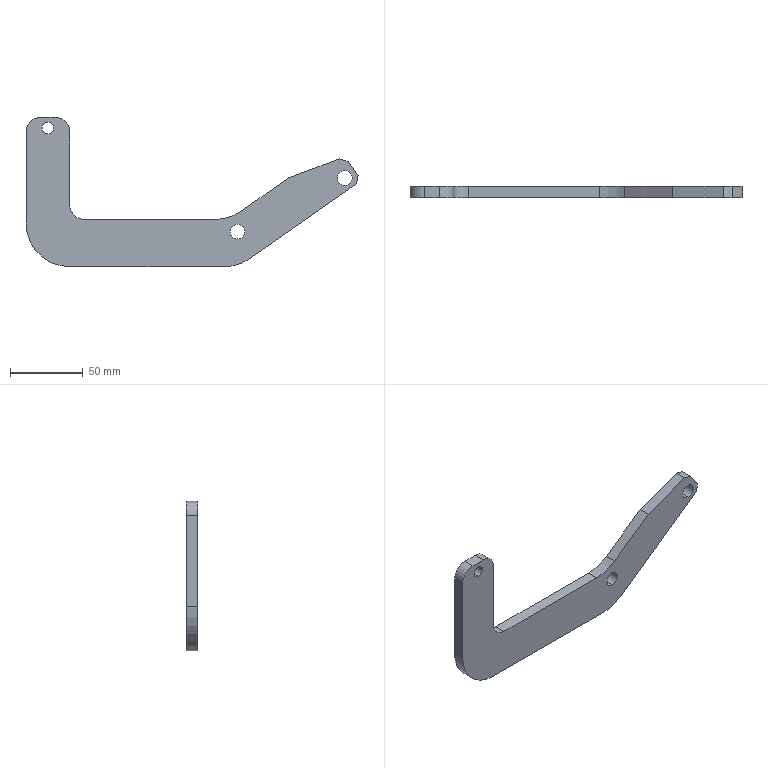Part | SolidWorks | features Extrusion 1, Fillet 1, ICE 1 | 1 solid | 25 faces | box 227.652 x 7.9 x 102.468 mm | volume 70886 mm3 | plane 13 | cylinder 12 | commonest cylinder face diameters 10 x4 20 x3 60 x3 8 x2
STEP:
#1=CARTESIAN_POINT('',(114.715,7.9,3.068));
#2=VERTEX_POINT('',#1);
#3=CARTESIAN_POINT('',(114.715,7.9,-6.932));
#4=VERTEX_POINT('',#3);
#5=CARTESIAN_POINT('',(114.715,7.9,-1.932));
#6=DIRECTION('',(0.,-1.,0.));
#7=DIRECTION('',(0.,0.,-1.));
#8=AXIS2_PLACEMENT_3D('',#5,#6,#7);
#9=CIRCLE('',#8,5.);
#10=EDGE_CURVE('',#2,#4,#9,.T.);
#11=ORIENTED_EDGE('',*,*,#10,.F.);
#12=CARTESIAN_POINT('',(114.715,0.,3.068));
#13=VERTEX_POINT('',#12);
#14=CARTESIAN_POINT('',(114.715,7.9,3.068));
#15=DIRECTION('',(0.,-1.,0.));
#16=VECTOR('',#15,1000.);
#17=LINE('',#14,#16);
#18=EDGE_CURVE('',#2,#13,#17,.T.);
#19=ORIENTED_EDGE('',*,*,#18,.T.);
#20=CARTESIAN_POINT('',(114.715,0.,-6.932));
#21=VERTEX_POINT('',#20);
#22=CARTESIAN_POINT('',(114.715,0.,-1.932));
#23=DIRECTION('',(0.,-1.,0.));
#24=DIRECTION('',(0.,0.,-1.));
#25=AXIS2_PLACEMENT_3D('',#22,#23,#24);
#26=CIRCLE('',#25,5.);
#27=EDGE_CURVE('',#13,#21,#26,.T.);
#28=ORIENTED_EDGE('',*,*,#27,.T.);
#29=CARTESIAN_POINT('',(114.715,7.9,-6.932));
#30=DIRECTION('',(0.,-1.,0.));
#31=VECTOR('',#30,1000.);
#32=LINE('',#29,#31);
#33=EDGE_CURVE('',#4,#21,#32,.T.);
#34=ORIENTED_EDGE('',*,*,#33,.F.);
#35=EDGE_LOOP('',(#11,#19,#28,#34));
#36=FACE_OUTER_BOUND('',#35,.T.);
#37=CARTESIAN_POINT('',(114.715,7.9,-1.932));
#38=DIRECTION('',(0.,-1.,0.));
#39=DIRECTION('',(0.,0.,-1.));
#40=AXIS2_PLACEMENT_3D('',#37,#38,#39);
#41=CYLINDRICAL_SURFACE('',#40,5.);
#42=ADVANCED_FACE('',(#36),#41,.F.);
#43=CARTESIAN_POINT('',(-15.275,7.9,65.119));
#44=VERTEX_POINT('',#43);
#45=CARTESIAN_POINT('',(-15.275,7.9,73.119));
#46=VERTEX_POINT('',#45);
#47=CARTESIAN_POINT('',(-15.275,7.9,69.119));
#48=DIRECTION('',(0.,1.,0.));
#49=DIRECTION('',(0.,0.,1.));
#50=AXIS2_PLACEMENT_3D('',#47,#48,#49);
#51=CIRCLE('',#50,4.);
#52=EDGE_CURVE('',#44,#46,#51,.T.);
#53=ORIENTED_EDGE('',*,*,#52,.T.);
#54=CARTESIAN_POINT('',(-15.275,0.,73.119));
#55=VERTEX_POINT('',#54);
#56=CARTESIAN_POINT('',(-15.275,7.9,73.119));
#57=DIRECTION('',(0.,-1.,0.));
#58=VECTOR('',#57,1000.);
#59=LINE('',#56,#58);
#60=EDGE_CURVE('',#46,#55,#59,.T.);
#61=ORIENTED_EDGE('',*,*,#60,.T.);
#62=CARTESIAN_POINT('',(-15.275,0.,65.119));
#63=VERTEX_POINT('',#62);
#64=CARTESIAN_POINT('',(-15.275,0.,69.119));
#65=DIRECTION('',(0.,1.,0.));
#66=DIRECTION('',(0.,0.,1.));
#67=AXIS2_PLACEMENT_3D('',#64,#65,#66);
#68=CIRCLE('',#67,4.);
#69=EDGE_CURVE('',#63,#55,#68,.T.);
#70=ORIENTED_EDGE('',*,*,#69,.F.);
#71=CARTESIAN_POINT('',(-15.275,7.9,65.119));
#72=DIRECTION('',(0.,-1.,0.));
#73=VECTOR('',#72,1000.);
#74=LINE('',#71,#73);
#75=EDGE_CURVE('',#44,#63,#74,.T.);
#76=ORIENTED_EDGE('',*,*,#75,.F.);
#77=EDGE_LOOP('',(#53,#61,#70,#76));
#78=FACE_OUTER_BOUND('',#77,.T.);
#79=CARTESIAN_POINT('',(-15.275,7.9,69.119));
#80=DIRECTION('',(0.,-1.,0.));
#81=DIRECTION('',(0.,0.,-1.));
#82=AXIS2_PLACEMENT_3D('',#79,#80,#81);
#83=CYLINDRICAL_SURFACE('',#82,4.);
#84=ADVANCED_FACE('',(#78),#83,.F.);
#85=CARTESIAN_POINT('',(188.312,7.9,29.854));
#86=VERTEX_POINT('',#85);
#87=CARTESIAN_POINT('',(188.312,7.9,39.854));
#88=VERTEX_POINT('',#87);
#89=CARTESIAN_POINT('',(188.312,7.9,34.854));
#90=DIRECTION('',(0.,1.,0.));
#91=DIRECTION('',(0.,0.,1.));
#92=AXIS2_PLACEMENT_3D('',#89,#90,#91);
#93=CIRCLE('',#92,5.);
#94=EDGE_CURVE('',#86,#88,#93,.T.);
#95=ORIENTED_EDGE('',*,*,#94,.T.);
#96=CARTESIAN_POINT('',(188.312,0.,39.854));
#97=VERTEX_POINT('',#96);
#98=CARTESIAN_POINT('',(188.312,7.9,39.854));
#99=DIRECTION('',(0.,-1.,0.));
#100=VECTOR('',#99,1000.);
#101=LINE('',#98,#100);
#102=EDGE_CURVE('',#88,#97,#101,.T.);
#103=ORIENTED_EDGE('',*,*,#102,.T.);
#104=CARTESIAN_POINT('',(188.312,0.,29.854));
#105=VERTEX_POINT('',#104);
#106=CARTESIAN_POINT('',(188.312,0.,34.854));
#107=DIRECTION('',(0.,1.,0.));
#108=DIRECTION('',(0.,0.,1.));
#109=AXIS2_PLACEMENT_3D('',#106,#107,#108);
#110=CIRCLE('',#109,5.);
#111=EDGE_CURVE('',#105,#97,#110,.T.);
#112=ORIENTED_EDGE('',*,*,#111,.F.);
#113=CARTESIAN_POINT('',(188.312,7.9,29.854));
#114=DIRECTION('',(0.,-1.,0.));
#115=VECTOR('',#114,1000.);
#116=LINE('',#113,#115);
#117=EDGE_CURVE('',#86,#105,#116,.T.);
#118=ORIENTED_EDGE('',*,*,#117,.F.);
#119=EDGE_LOOP('',(#95,#103,#112,#118));
#120=FACE_OUTER_BOUND('',#119,.T.);
#121=CARTESIAN_POINT('',(188.312,7.9,34.854));
#122=DIRECTION('',(0.,-1.,0.));
#123=DIRECTION('',(0.,0.,-1.));
#124=AXIS2_PLACEMENT_3D('',#121,#122,#123);
#125=CYLINDRICAL_SURFACE('',#124,5.);
#126=ADVANCED_FACE('',(#120),#125,.F.);
#127=CARTESIAN_POINT('',(114.715,7.9,-1.932));
#128=DIRECTION('',(0.,-1.,0.));
#129=DIRECTION('',(0.,0.,-1.));
#130=AXIS2_PLACEMENT_3D('',#127,#128,#129);
#131=CIRCLE('',#130,5.);
#132=EDGE_CURVE('',#4,#2,#131,.T.);
#133=ORIENTED_EDGE('',*,*,#132,.T.);
#134=ORIENTED_EDGE('',*,*,#10,.T.);
#135=EDGE_LOOP('',(#133,#134));
#136=FACE_BOUND('',#135,.T.);
#137=CARTESIAN_POINT('',(-20.275,7.9,76.485));
#138=VERTEX_POINT('',#137);
#139=CARTESIAN_POINT('',(-10.275,7.9,76.485));
#140=VERTEX_POINT('',#139);
#141=CARTESIAN_POINT('',(-0.2746,7.9,76.485));
#142=DIRECTION('',(1.,0.,0.));
#143=VECTOR('',#142,1000.);
#144=LINE('',#141,#143);
#145=EDGE_CURVE('',#138,#140,#144,.T.);
#146=ORIENTED_EDGE('',*,*,#145,.T.);
#147=CARTESIAN_POINT('',(-0.2746,7.9,66.485));
#148=VERTEX_POINT('',#147);
#149=CARTESIAN_POINT('',(-10.275,7.9,66.485));
#150=DIRECTION('',(0.,1.,0.));
#151=DIRECTION('',(0.,0.,-1.));
#152=AXIS2_PLACEMENT_3D('',#149,#150,#151);
#153=CIRCLE('',#152,10.);
#154=EDGE_CURVE('',#140,#148,#153,.T.);
#155=ORIENTED_EDGE('',*,*,#154,.T.);
#156=CARTESIAN_POINT('',(-0.2746,7.9,16.485));
#157=VERTEX_POINT('',#156);
#158=CARTESIAN_POINT('',(-0.2746,7.9,16.485));
#159=DIRECTION('',(0.,0.,-1.));
#160=VECTOR('',#159,1000.);
#161=LINE('',#158,#160);
#162=EDGE_CURVE('',#148,#157,#161,.T.);
#163=ORIENTED_EDGE('',*,*,#162,.T.);
#164=CARTESIAN_POINT('',(9.725,7.9,6.485));
#165=VERTEX_POINT('',#164);
#166=CARTESIAN_POINT('',(9.725,7.9,16.485));
#167=DIRECTION('',(0.,-1.,0.));
#168=DIRECTION('',(0.,0.,-1.));
#169=AXIS2_PLACEMENT_3D('',#166,#167,#168);
#170=CIRCLE('',#169,10.);
#171=EDGE_CURVE('',#157,#165,#170,.T.);
#172=ORIENTED_EDGE('',*,*,#171,.T.);
#173=CARTESIAN_POINT('',(99.725,7.9,6.485));
#174=VERTEX_POINT('',#173);
#175=CARTESIAN_POINT('',(99.725,7.9,6.485));
#176=DIRECTION('',(1.,0.,0.));
#177=VECTOR('',#176,1000.);
#178=LINE('',#175,#177);
#179=EDGE_CURVE('',#165,#174,#178,.T.);
#180=ORIENTED_EDGE('',*,*,#179,.T.);
#181=CARTESIAN_POINT('',(116.933,7.9,11.91));
#182=VERTEX_POINT('',#181);
#183=CARTESIAN_POINT('',(99.725,7.9,36.485));
#184=DIRECTION('',(0.,-1.,0.));
#185=DIRECTION('',(0.,0.,1.));
#186=AXIS2_PLACEMENT_3D('',#183,#184,#185);
#187=CIRCLE('',#186,30.);
#188=EDGE_CURVE('',#174,#182,#187,.T.);
#189=ORIENTED_EDGE('',*,*,#188,.T.);
#190=CARTESIAN_POINT('',(149.699,7.9,34.854));
#191=VERTEX_POINT('',#190);
#192=CARTESIAN_POINT('',(149.699,7.9,34.854));
#193=DIRECTION('',(0.8192,0.,0.5736));
#194=VECTOR('',#193,1000.);
#195=LINE('',#192,#194);
#196=EDGE_CURVE('',#182,#191,#195,.T.);
#197=ORIENTED_EDGE('',*,*,#196,.T.);
#198=CARTESIAN_POINT('',(184.57,7.9,48.032));
#199=VERTEX_POINT('',#198);
#200=CARTESIAN_POINT('',(184.57,7.9,48.032));
#201=DIRECTION('',(0.9354,0.,0.3535));
#202=VECTOR('',#201,1000.);
#203=LINE('',#200,#202);
#204=EDGE_CURVE('',#191,#199,#203,.T.);
#205=ORIENTED_EDGE('',*,*,#204,.T.);
#206=CARTESIAN_POINT('',(190.606,7.9,46.169));
#207=VERTEX_POINT('',#206);
#208=CARTESIAN_POINT('',(190.606,7.9,46.169));
#209=DIRECTION('',(0.9555,0.,-0.2949));
#210=VECTOR('',#209,1000.);
#211=LINE('',#208,#210);
#212=EDGE_CURVE('',#199,#207,#211,.T.);
#213=ORIENTED_EDGE('',*,*,#212,.T.);
#214=CARTESIAN_POINT('',(197.378,7.9,36.499));
#215=VERTEX_POINT('',#214);
#216=CARTESIAN_POINT('',(197.378,7.9,36.499));
#217=DIRECTION('',(0.5736,0.,-0.8192));
#218=VECTOR('',#217,1000.);
#219=LINE('',#216,#218);
#220=EDGE_CURVE('',#207,#215,#219,.T.);
#221=ORIENTED_EDGE('',*,*,#220,.T.);
#222=CARTESIAN_POINT('',(196.396,7.9,30.928));
#223=VERTEX_POINT('',#222);
#224=CARTESIAN_POINT('',(197.378,7.9,36.499));
#225=DIRECTION('',(-0.1736,0.,-0.9848));
#226=VECTOR('',#225,1000.);
#227=LINE('',#224,#226);
#228=EDGE_CURVE('',#215,#223,#227,.T.);
#229=ORIENTED_EDGE('',*,*,#228,.T.);
#230=CARTESIAN_POINT('',(122.867,7.9,-20.557));
#231=VERTEX_POINT('',#230);
#232=CARTESIAN_POINT('',(196.396,7.9,30.928));
#233=DIRECTION('',(-0.8192,0.,-0.5736));
#234=VECTOR('',#233,1000.);
#235=LINE('',#232,#234);
#236=EDGE_CURVE('',#223,#231,#235,.T.);
#237=ORIENTED_EDGE('',*,*,#236,.T.);
#238=CARTESIAN_POINT('',(105.66,7.9,-25.983));
#239=VERTEX_POINT('',#238);
#240=CARTESIAN_POINT('',(105.66,7.9,4.017));
#241=DIRECTION('',(0.,1.,0.));
#242=DIRECTION('',(0.,0.,1.));
#243=AXIS2_PLACEMENT_3D('',#240,#241,#242);
#244=CIRCLE('',#243,30.);
#245=EDGE_CURVE('',#231,#239,#244,.T.);
#246=ORIENTED_EDGE('',*,*,#245,.T.);
#247=CARTESIAN_POINT('',(-0.2746,7.9,-25.983));
#248=VERTEX_POINT('',#247);
#249=CARTESIAN_POINT('',(105.66,7.9,-25.983));
#250=DIRECTION('',(-1.,0.,0.));
#251=VECTOR('',#250,1000.);
#252=LINE('',#249,#251);
#253=EDGE_CURVE('',#239,#248,#252,.T.);
#254=ORIENTED_EDGE('',*,*,#253,.T.);
#255=CARTESIAN_POINT('',(-30.275,7.9,4.017));
#256=VERTEX_POINT('',#255);
#257=CARTESIAN_POINT('',(-0.2746,7.9,4.017));
#258=DIRECTION('',(0.,1.,0.));
#259=DIRECTION('',(0.,0.,-1.));
#260=AXIS2_PLACEMENT_3D('',#257,#258,#259);
#261=CIRCLE('',#260,30.);
#262=EDGE_CURVE('',#248,#256,#261,.T.);
#263=ORIENTED_EDGE('',*,*,#262,.T.);
#264=CARTESIAN_POINT('',(-30.275,7.9,66.485));
#265=VERTEX_POINT('',#264);
#266=CARTESIAN_POINT('',(-30.275,7.9,76.485));
#267=DIRECTION('',(0.,0.,1.));
#268=VECTOR('',#267,1000.);
#269=LINE('',#266,#268);
#270=EDGE_CURVE('',#256,#265,#269,.T.);
#271=ORIENTED_EDGE('',*,*,#270,.T.);
#272=CARTESIAN_POINT('',(-20.275,7.9,66.485));
#273=DIRECTION('',(0.,1.,0.));
#274=DIRECTION('',(0.,0.,-1.));
#275=AXIS2_PLACEMENT_3D('',#272,#273,#274);
#276=CIRCLE('',#275,10.);
#277=EDGE_CURVE('',#265,#138,#276,.T.);
#278=ORIENTED_EDGE('',*,*,#277,.T.);
#279=EDGE_LOOP('',(#146,#155,#163,#172,#180,#189,#197,#205,#213,#221,#229,#237,#246,#254,#263,#271,#278));
#280=FACE_OUTER_BOUND('',#279,.T.);
#281=ORIENTED_EDGE('',*,*,#94,.F.);
#282=CARTESIAN_POINT('',(188.312,7.9,34.854));
#283=DIRECTION('',(0.,1.,0.));
#284=DIRECTION('',(0.,0.,1.));
#285=AXIS2_PLACEMENT_3D('',#282,#283,#284);
#286=CIRCLE('',#285,5.);
#287=EDGE_CURVE('',#88,#86,#286,.T.);
#288=ORIENTED_EDGE('',*,*,#287,.F.);
#289=EDGE_LOOP('',(#281,#288));
#290=FACE_BOUND('',#289,.T.);
#291=ORIENTED_EDGE('',*,*,#52,.F.);
#292=CARTESIAN_POINT('',(-15.275,7.9,69.119));
#293=DIRECTION('',(0.,1.,0.));
#294=DIRECTION('',(0.,0.,1.));
#295=AXIS2_PLACEMENT_3D('',#292,#293,#294);
#296=CIRCLE('',#295,4.);
#297=EDGE_CURVE('',#46,#44,#296,.T.);
#298=ORIENTED_EDGE('',*,*,#297,.F.);
#299=EDGE_LOOP('',(#291,#298));
#300=FACE_BOUND('',#299,.T.);
#301=CARTESIAN_POINT('',(-0.2746,7.9,4.017));
#302=DIRECTION('',(0.,-1.,0.));
#303=DIRECTION('',(0.,0.,-1.));
#304=AXIS2_PLACEMENT_3D('',#301,#302,#303);
#305=PLANE('',#304);
#306=ADVANCED_FACE('',(#136,#280,#290,#300),#305,.F.);
#307=CARTESIAN_POINT('',(114.715,0.,-1.932));
#308=DIRECTION('',(0.,-1.,0.));
#309=DIRECTION('',(0.,0.,-1.));
#310=AXIS2_PLACEMENT_3D('',#307,#308,#309);
#311=CIRCLE('',#310,5.);
#312=EDGE_CURVE('',#21,#13,#311,.T.);
#313=ORIENTED_EDGE('',*,*,#312,.F.);
#314=ORIENTED_EDGE('',*,*,#27,.F.);
#315=EDGE_LOOP('',(#313,#314));
#316=FACE_BOUND('',#315,.T.);
#317=ORIENTED_EDGE('',*,*,#111,.T.);
#318=CARTESIAN_POINT('',(188.312,0.,34.854));
#319=DIRECTION('',(0.,1.,0.));
#320=DIRECTION('',(0.,0.,1.));
#321=AXIS2_PLACEMENT_3D('',#318,#319,#320);
#322=CIRCLE('',#321,5.);
#323=EDGE_CURVE('',#97,#105,#322,.T.);
#324=ORIENTED_EDGE('',*,*,#323,.T.);
#325=EDGE_LOOP('',(#317,#324));
#326=FACE_BOUND('',#325,.T.);
#327=CARTESIAN_POINT('',(-0.2746,0.,66.485));
#328=VERTEX_POINT('',#327);
#329=CARTESIAN_POINT('',(-0.2746,0.,16.485));
#330=VERTEX_POINT('',#329);
#331=CARTESIAN_POINT('',(-0.2746,0.,16.485));
#332=DIRECTION('',(0.,0.,-1.));
#333=VECTOR('',#332,1000.);
#334=LINE('',#331,#333);
#335=EDGE_CURVE('',#328,#330,#334,.T.);
#336=ORIENTED_EDGE('',*,*,#335,.F.);
#337=CARTESIAN_POINT('',(-10.275,0.,76.485));
#338=VERTEX_POINT('',#337);
#339=CARTESIAN_POINT('',(-10.275,0.,66.485));
#340=DIRECTION('',(0.,-1.,0.));
#341=DIRECTION('',(0.,0.,-1.));
#342=AXIS2_PLACEMENT_3D('',#339,#340,#341);
#343=CIRCLE('',#342,10.);
#344=EDGE_CURVE('',#328,#338,#343,.T.);
#345=ORIENTED_EDGE('',*,*,#344,.T.);
#346=CARTESIAN_POINT('',(-20.275,0.,76.485));
#347=VERTEX_POINT('',#346);
#348=CARTESIAN_POINT('',(-0.2746,0.,76.485));
#349=DIRECTION('',(1.,0.,0.));
#350=VECTOR('',#349,1000.);
#351=LINE('',#348,#350);
#352=EDGE_CURVE('',#347,#338,#351,.T.);
#353=ORIENTED_EDGE('',*,*,#352,.F.);
#354=CARTESIAN_POINT('',(-30.275,0.,66.485));
#355=VERTEX_POINT('',#354);
#356=CARTESIAN_POINT('',(-20.275,0.,66.485));
#357=DIRECTION('',(0.,-1.,0.));
#358=DIRECTION('',(0.,0.,-1.));
#359=AXIS2_PLACEMENT_3D('',#356,#357,#358);
#360=CIRCLE('',#359,10.);
#361=EDGE_CURVE('',#347,#355,#360,.T.);
#362=ORIENTED_EDGE('',*,*,#361,.T.);
#363=CARTESIAN_POINT('',(-30.275,0.,4.017));
#364=VERTEX_POINT('',#363);
#365=CARTESIAN_POINT('',(-30.275,0.,76.485));
#366=DIRECTION('',(0.,0.,1.));
#367=VECTOR('',#366,1000.);
#368=LINE('',#365,#367);
#369=EDGE_CURVE('',#364,#355,#368,.T.);
#370=ORIENTED_EDGE('',*,*,#369,.F.);
#371=CARTESIAN_POINT('',(-0.2746,0.,-25.983));
#372=VERTEX_POINT('',#371);
#373=CARTESIAN_POINT('',(-0.2746,0.,4.017));
#374=DIRECTION('',(0.,1.,0.));
#375=DIRECTION('',(0.,0.,-1.));
#376=AXIS2_PLACEMENT_3D('',#373,#374,#375);
#377=CIRCLE('',#376,30.);
#378=EDGE_CURVE('',#372,#364,#377,.T.);
#379=ORIENTED_EDGE('',*,*,#378,.F.);
#380=CARTESIAN_POINT('',(105.66,0.,-25.983));
#381=VERTEX_POINT('',#380);
#382=CARTESIAN_POINT('',(105.66,0.,-25.983));
#383=DIRECTION('',(-1.,0.,0.));
#384=VECTOR('',#383,1000.);
#385=LINE('',#382,#384);
#386=EDGE_CURVE('',#381,#372,#385,.T.);
#387=ORIENTED_EDGE('',*,*,#386,.F.);
#388=CARTESIAN_POINT('',(122.867,0.,-20.557));
#389=VERTEX_POINT('',#388);
#390=CARTESIAN_POINT('',(105.66,0.,4.017));
#391=DIRECTION('',(0.,1.,0.));
#392=DIRECTION('',(0.,0.,1.));
#393=AXIS2_PLACEMENT_3D('',#390,#391,#392);
#394=CIRCLE('',#393,30.);
#395=EDGE_CURVE('',#389,#381,#394,.T.);
#396=ORIENTED_EDGE('',*,*,#395,.F.);
#397=CARTESIAN_POINT('',(196.396,0.,30.928));
#398=VERTEX_POINT('',#397);
#399=CARTESIAN_POINT('',(196.396,0.,30.928));
#400=DIRECTION('',(-0.8192,0.,-0.5736));
#401=VECTOR('',#400,1000.);
#402=LINE('',#399,#401);
#403=EDGE_CURVE('',#398,#389,#402,.T.);
#404=ORIENTED_EDGE('',*,*,#403,.F.);
#405=CARTESIAN_POINT('',(197.378,0.,36.499));
#406=VERTEX_POINT('',#405);
#407=CARTESIAN_POINT('',(197.378,0.,36.499));
#408=DIRECTION('',(-0.1736,0.,-0.9848));
#409=VECTOR('',#408,1000.);
#410=LINE('',#407,#409);
#411=EDGE_CURVE('',#406,#398,#410,.T.);
#412=ORIENTED_EDGE('',*,*,#411,.F.);
#413=CARTESIAN_POINT('',(190.606,0.,46.169));
#414=VERTEX_POINT('',#413);
#415=CARTESIAN_POINT('',(197.378,0.,36.499));
#416=DIRECTION('',(0.5736,0.,-0.8192));
#417=VECTOR('',#416,1000.);
#418=LINE('',#415,#417);
#419=EDGE_CURVE('',#414,#406,#418,.T.);
#420=ORIENTED_EDGE('',*,*,#419,.F.);
#421=CARTESIAN_POINT('',(184.57,0.,48.032));
#422=VERTEX_POINT('',#421);
#423=CARTESIAN_POINT('',(190.606,0.,46.169));
#424=DIRECTION('',(0.9555,0.,-0.2949));
#425=VECTOR('',#424,1000.);
#426=LINE('',#423,#425);
#427=EDGE_CURVE('',#422,#414,#426,.T.);
#428=ORIENTED_EDGE('',*,*,#427,.F.);
#429=CARTESIAN_POINT('',(149.699,0.,34.854));
#430=VERTEX_POINT('',#429);
#431=CARTESIAN_POINT('',(184.57,0.,48.032));
#432=DIRECTION('',(0.9354,0.,0.3535));
#433=VECTOR('',#432,1000.);
#434=LINE('',#431,#433);
#435=EDGE_CURVE('',#430,#422,#434,.T.);
#436=ORIENTED_EDGE('',*,*,#435,.F.);
#437=CARTESIAN_POINT('',(116.933,0.,11.91));
#438=VERTEX_POINT('',#437);
#439=CARTESIAN_POINT('',(149.699,0.,34.854));
#440=DIRECTION('',(0.8192,0.,0.5736));
#441=VECTOR('',#440,1000.);
#442=LINE('',#439,#441);
#443=EDGE_CURVE('',#438,#430,#442,.T.);
#444=ORIENTED_EDGE('',*,*,#443,.F.);
#445=CARTESIAN_POINT('',(99.725,0.,6.485));
#446=VERTEX_POINT('',#445);
#447=CARTESIAN_POINT('',(99.725,0.,36.485));
#448=DIRECTION('',(0.,-1.,0.));
#449=DIRECTION('',(0.,0.,1.));
#450=AXIS2_PLACEMENT_3D('',#447,#448,#449);
#451=CIRCLE('',#450,30.);
#452=EDGE_CURVE('',#446,#438,#451,.T.);
#453=ORIENTED_EDGE('',*,*,#452,.F.);
#454=CARTESIAN_POINT('',(9.725,0.,6.485));
#455=VERTEX_POINT('',#454);
#456=CARTESIAN_POINT('',(99.725,0.,6.485));
#457=DIRECTION('',(1.,0.,0.));
#458=VECTOR('',#457,1000.);
#459=LINE('',#456,#458);
#460=EDGE_CURVE('',#455,#446,#459,.T.);
#461=ORIENTED_EDGE('',*,*,#460,.F.);
#462=CARTESIAN_POINT('',(9.725,0.,16.485));
#463=DIRECTION('',(0.,-1.,0.));
#464=DIRECTION('',(0.,0.,-1.));
#465=AXIS2_PLACEMENT_3D('',#462,#463,#464);
#466=CIRCLE('',#465,10.);
#467=EDGE_CURVE('',#330,#455,#466,.T.);
#468=ORIENTED_EDGE('',*,*,#467,.F.);
#469=EDGE_LOOP('',(#336,#345,#353,#362,#370,#379,#387,#396,#404,#412,#420,#428,#436,#444,#453,#461,#468));
#470=FACE_OUTER_BOUND('',#469,.T.);
#471=ORIENTED_EDGE('',*,*,#69,.T.);
#472=CARTESIAN_POINT('',(-15.275,0.,69.119));
#473=DIRECTION('',(0.,1.,0.));
#474=DIRECTION('',(0.,0.,1.));
#475=AXIS2_PLACEMENT_3D('',#472,#473,#474);
#476=CIRCLE('',#475,4.);
#477=EDGE_CURVE('',#55,#63,#476,.T.);
#478=ORIENTED_EDGE('',*,*,#477,.T.);
#479=EDGE_LOOP('',(#471,#478));
#480=FACE_BOUND('',#479,.T.);
#481=CARTESIAN_POINT('',(-0.2746,0.,4.017));
#482=DIRECTION('',(0.,-1.,0.));
#483=DIRECTION('',(0.,0.,-1.));
#484=AXIS2_PLACEMENT_3D('',#481,#482,#483);
#485=PLANE('',#484);
#486=ADVANCED_FACE('',(#316,#326,#470,#480),#485,.T.);
#487=ORIENTED_EDGE('',*,*,#352,.T.);
#488=CARTESIAN_POINT('',(-10.275,7.9,76.485));
#489=DIRECTION('',(0.,1.,0.));
#490=VECTOR('',#489,1000.);
#491=LINE('',#488,#490);
#492=EDGE_CURVE('',#338,#140,#491,.T.);
#493=ORIENTED_EDGE('',*,*,#492,.T.);
#494=ORIENTED_EDGE('',*,*,#145,.F.);
#495=CARTESIAN_POINT('',(-20.275,7.9,76.485));
#496=DIRECTION('',(0.,-1.,0.));
#497=VECTOR('',#496,1000.);
#498=LINE('',#495,#497);
#499=EDGE_CURVE('',#138,#347,#498,.T.);
#500=ORIENTED_EDGE('',*,*,#499,.T.);
#501=EDGE_LOOP('',(#487,#493,#494,#500));
#502=FACE_OUTER_BOUND('',#501,.T.);
#503=CARTESIAN_POINT('',(-0.2746,7.9,76.485));
#504=DIRECTION('',(0.,0.,-1.));
#505=DIRECTION('',(-1.,0.,0.));
#506=AXIS2_PLACEMENT_3D('',#503,#504,#505);
#507=PLANE('',#506);
#508=ADVANCED_FACE('',(#502),#507,.F.);
#509=ORIENTED_EDGE('',*,*,#162,.F.);
#510=CARTESIAN_POINT('',(-0.2746,7.9,66.485));
#511=DIRECTION('',(0.,-1.,0.));
#512=VECTOR('',#511,1000.);
#513=LINE('',#510,#512);
#514=EDGE_CURVE('',#148,#328,#513,.T.);
#515=ORIENTED_EDGE('',*,*,#514,.T.);
#516=ORIENTED_EDGE('',*,*,#335,.T.);
#517=CARTESIAN_POINT('',(-0.2746,7.9,16.485));
#518=DIRECTION('',(0.,-1.,0.));
#519=VECTOR('',#518,1000.);
#520=LINE('',#517,#519);
#521=EDGE_CURVE('',#157,#330,#520,.T.);
#522=ORIENTED_EDGE('',*,*,#521,.F.);
#523=EDGE_LOOP('',(#509,#515,#516,#522));
#524=FACE_OUTER_BOUND('',#523,.T.);
#525=CARTESIAN_POINT('',(-0.2746,7.9,16.485));
#526=DIRECTION('',(-1.,0.,0.));
#527=DIRECTION('',(0.,0.,1.));
#528=AXIS2_PLACEMENT_3D('',#525,#526,#527);
#529=PLANE('',#528);
#530=ADVANCED_FACE('',(#524),#529,.F.);
#531=ORIENTED_EDGE('',*,*,#467,.T.);
#532=CARTESIAN_POINT('',(9.725,7.9,6.485));
#533=DIRECTION('',(0.,-1.,0.));
#534=VECTOR('',#533,1000.);
#535=LINE('',#532,#534);
#536=EDGE_CURVE('',#165,#455,#535,.T.);
#537=ORIENTED_EDGE('',*,*,#536,.F.);
#538=ORIENTED_EDGE('',*,*,#171,.F.);
#539=ORIENTED_EDGE('',*,*,#521,.T.);
#540=EDGE_LOOP('',(#531,#537,#538,#539));
#541=FACE_OUTER_BOUND('',#540,.T.);
#542=CARTESIAN_POINT('',(9.725,7.9,16.485));
#543=DIRECTION('',(0.,-1.,0.));
#544=DIRECTION('',(0.,0.,-1.));
#545=AXIS2_PLACEMENT_3D('',#542,#543,#544);
#546=CYLINDRICAL_SURFACE('',#545,10.);
#547=ADVANCED_FACE('',(#541),#546,.F.);
#548=ORIENTED_EDGE('',*,*,#460,.T.);
#549=CARTESIAN_POINT('',(99.725,7.9,6.485));
#550=DIRECTION('',(0.,-1.,0.));
#551=VECTOR('',#550,1000.);
#552=LINE('',#549,#551);
#553=EDGE_CURVE('',#174,#446,#552,.T.);
#554=ORIENTED_EDGE('',*,*,#553,.F.);
#555=ORIENTED_EDGE('',*,*,#179,.F.);
#556=ORIENTED_EDGE('',*,*,#536,.T.);
#557=EDGE_LOOP('',(#548,#554,#555,#556));
#558=FACE_OUTER_BOUND('',#557,.T.);
#559=CARTESIAN_POINT('',(99.725,7.9,6.485));
#560=DIRECTION('',(0.,0.,-1.));
#561=DIRECTION('',(-1.,0.,0.));
#562=AXIS2_PLACEMENT_3D('',#559,#560,#561);
#563=PLANE('',#562);
#564=ADVANCED_FACE('',(#558),#563,.F.);
#565=ORIENTED_EDGE('',*,*,#452,.T.);
#566=CARTESIAN_POINT('',(116.933,7.9,11.91));
#567=DIRECTION('',(0.,-1.,0.));
#568=VECTOR('',#567,1000.);
#569=LINE('',#566,#568);
#570=EDGE_CURVE('',#182,#438,#569,.T.);
#571=ORIENTED_EDGE('',*,*,#570,.F.);
#572=ORIENTED_EDGE('',*,*,#188,.F.);
#573=ORIENTED_EDGE('',*,*,#553,.T.);
#574=EDGE_LOOP('',(#565,#571,#572,#573));
#575=FACE_OUTER_BOUND('',#574,.T.);
#576=CARTESIAN_POINT('',(99.725,7.9,36.485));
#577=DIRECTION('',(0.,-1.,0.));
#578=DIRECTION('',(0.,0.,-1.));
#579=AXIS2_PLACEMENT_3D('',#576,#577,#578);
#580=CYLINDRICAL_SURFACE('',#579,30.);
#581=ADVANCED_FACE('',(#575),#580,.F.);
#582=ORIENTED_EDGE('',*,*,#443,.T.);
#583=CARTESIAN_POINT('',(149.699,7.9,34.854));
#584=DIRECTION('',(0.,-1.,0.));
#585=VECTOR('',#584,1000.);
#586=LINE('',#583,#585);
#587=EDGE_CURVE('',#191,#430,#586,.T.);
#588=ORIENTED_EDGE('',*,*,#587,.F.);
#589=ORIENTED_EDGE('',*,*,#196,.F.);
#590=ORIENTED_EDGE('',*,*,#570,.T.);
#591=EDGE_LOOP('',(#582,#588,#589,#590));
#592=FACE_OUTER_BOUND('',#591,.T.);
#593=CARTESIAN_POINT('',(149.699,7.9,34.854));
#594=DIRECTION('',(0.5736,0.,-0.8192));
#595=DIRECTION('',(-0.8192,0.,-0.5736));
#596=AXIS2_PLACEMENT_3D('',#593,#594,#595);
#597=PLANE('',#596);
#598=ADVANCED_FACE('',(#592),#597,.F.);
#599=ORIENTED_EDGE('',*,*,#435,.T.);
#600=CARTESIAN_POINT('',(184.57,7.9,48.032));
#601=DIRECTION('',(0.,-1.,0.));
#602=VECTOR('',#601,1000.);
#603=LINE('',#600,#602);
#604=EDGE_CURVE('',#199,#422,#603,.T.);
#605=ORIENTED_EDGE('',*,*,#604,.F.);
#606=ORIENTED_EDGE('',*,*,#204,.F.);
#607=ORIENTED_EDGE('',*,*,#587,.T.);
#608=EDGE_LOOP('',(#599,#605,#606,#607));
#609=FACE_OUTER_BOUND('',#608,.T.);
#610=CARTESIAN_POINT('',(184.57,7.9,48.032));
#611=DIRECTION('',(0.3535,0.,-0.9354));
#612=DIRECTION('',(-0.9354,0.,-0.3535));
#613=AXIS2_PLACEMENT_3D('',#610,#611,#612);
#614=PLANE('',#613);
#615=ADVANCED_FACE('',(#609),#614,.F.);
#616=ORIENTED_EDGE('',*,*,#427,.T.);
#617=CARTESIAN_POINT('',(190.606,7.9,46.169));
#618=DIRECTION('',(0.,-1.,0.));
#619=VECTOR('',#618,1000.);
#620=LINE('',#617,#619);
#621=EDGE_CURVE('',#207,#414,#620,.T.);
#622=ORIENTED_EDGE('',*,*,#621,.F.);
#623=ORIENTED_EDGE('',*,*,#212,.F.);
#624=ORIENTED_EDGE('',*,*,#604,.T.);
#625=EDGE_LOOP('',(#616,#622,#623,#624));
#626=FACE_OUTER_BOUND('',#625,.T.);
#627=CARTESIAN_POINT('',(190.606,7.9,46.169));
#628=DIRECTION('',(-0.2949,0.,-0.9555));
#629=DIRECTION('',(-0.9555,0.,0.2949));
#630=AXIS2_PLACEMENT_3D('',#627,#628,#629);
#631=PLANE('',#630);
#632=ADVANCED_FACE('',(#626),#631,.F.);
#633=ORIENTED_EDGE('',*,*,#419,.T.);
#634=CARTESIAN_POINT('',(197.378,7.9,36.499));
#635=DIRECTION('',(0.,-1.,0.));
#636=VECTOR('',#635,1000.);
#637=LINE('',#634,#636);
#638=EDGE_CURVE('',#215,#406,#637,.T.);
#639=ORIENTED_EDGE('',*,*,#638,.F.);
#640=ORIENTED_EDGE('',*,*,#220,.F.);
#641=ORIENTED_EDGE('',*,*,#621,.T.);
#642=EDGE_LOOP('',(#633,#639,#640,#641));
#643=FACE_OUTER_BOUND('',#642,.T.);
#644=CARTESIAN_POINT('',(197.378,7.9,36.499));
#645=DIRECTION('',(-0.8192,0.,-0.5736));
#646=DIRECTION('',(-0.5736,0.,0.8192));
#647=AXIS2_PLACEMENT_3D('',#644,#645,#646);
#648=PLANE('',#647);
#649=ADVANCED_FACE('',(#643),#648,.F.);
#650=ORIENTED_EDGE('',*,*,#411,.T.);
#651=CARTESIAN_POINT('',(196.396,7.9,30.928));
#652=DIRECTION('',(0.,-1.,0.));
#653=VECTOR('',#652,1000.);
#654=LINE('',#651,#653);
#655=EDGE_CURVE('',#223,#398,#654,.T.);
#656=ORIENTED_EDGE('',*,*,#655,.F.);
#657=ORIENTED_EDGE('',*,*,#228,.F.);
#658=ORIENTED_EDGE('',*,*,#638,.T.);
#659=EDGE_LOOP('',(#650,#656,#657,#658));
#660=FACE_OUTER_BOUND('',#659,.T.);
#661=CARTESIAN_POINT('',(197.378,7.9,36.499));
#662=DIRECTION('',(-0.9848,0.,0.1736));
#663=DIRECTION('',(0.1736,0.,0.9848));
#664=AXIS2_PLACEMENT_3D('',#661,#662,#663);
#665=PLANE('',#664);
#666=ADVANCED_FACE('',(#660),#665,.F.);
#667=ORIENTED_EDGE('',*,*,#403,.T.);
#668=CARTESIAN_POINT('',(122.867,7.9,-20.557));
#669=DIRECTION('',(0.,-1.,0.));
#670=VECTOR('',#669,1000.);
#671=LINE('',#668,#670);
#672=EDGE_CURVE('',#231,#389,#671,.T.);
#673=ORIENTED_EDGE('',*,*,#672,.F.);
#674=ORIENTED_EDGE('',*,*,#236,.F.);
#675=ORIENTED_EDGE('',*,*,#655,.T.);
#676=EDGE_LOOP('',(#667,#673,#674,#675));
#677=FACE_OUTER_BOUND('',#676,.T.);
#678=CARTESIAN_POINT('',(196.396,7.9,30.928));
#679=DIRECTION('',(-0.5736,0.,0.8192));
#680=DIRECTION('',(0.8192,0.,0.5736));
#681=AXIS2_PLACEMENT_3D('',#678,#679,#680);
#682=PLANE('',#681);
#683=ADVANCED_FACE('',(#677),#682,.F.);
#684=ORIENTED_EDGE('',*,*,#395,.T.);
#685=CARTESIAN_POINT('',(105.66,7.9,-25.983));
#686=DIRECTION('',(0.,-1.,0.));
#687=VECTOR('',#686,1000.);
#688=LINE('',#685,#687);
#689=EDGE_CURVE('',#239,#381,#688,.T.);
#690=ORIENTED_EDGE('',*,*,#689,.F.);
#691=ORIENTED_EDGE('',*,*,#245,.F.);
#692=ORIENTED_EDGE('',*,*,#672,.T.);
#693=EDGE_LOOP('',(#684,#690,#691,#692));
#694=FACE_OUTER_BOUND('',#693,.T.);
#695=CARTESIAN_POINT('',(105.66,7.9,4.017));
#696=DIRECTION('',(0.,-1.,0.));
#697=DIRECTION('',(0.,0.,-1.));
#698=AXIS2_PLACEMENT_3D('',#695,#696,#697);
#699=CYLINDRICAL_SURFACE('',#698,30.);
#700=ADVANCED_FACE('',(#694),#699,.T.);
#701=ORIENTED_EDGE('',*,*,#386,.T.);
#702=CARTESIAN_POINT('',(-0.2746,7.9,-25.983));
#703=DIRECTION('',(0.,-1.,0.));
#704=VECTOR('',#703,1000.);
#705=LINE('',#702,#704);
#706=EDGE_CURVE('',#248,#372,#705,.T.);
#707=ORIENTED_EDGE('',*,*,#706,.F.);
#708=ORIENTED_EDGE('',*,*,#253,.F.);
#709=ORIENTED_EDGE('',*,*,#689,.T.);
#710=EDGE_LOOP('',(#701,#707,#708,#709));
#711=FACE_OUTER_BOUND('',#710,.T.);
#712=CARTESIAN_POINT('',(105.66,7.9,-25.983));
#713=DIRECTION('',(0.,0.,1.));
#714=DIRECTION('',(1.,0.,0.));
#715=AXIS2_PLACEMENT_3D('',#712,#713,#714);
#716=PLANE('',#715);
#717=ADVANCED_FACE('',(#711),#716,.F.);
#718=ORIENTED_EDGE('',*,*,#378,.T.);
#719=CARTESIAN_POINT('',(-30.275,7.9,4.017));
#720=DIRECTION('',(0.,-1.,0.));
#721=VECTOR('',#720,1000.);
#722=LINE('',#719,#721);
#723=EDGE_CURVE('',#256,#364,#722,.T.);
#724=ORIENTED_EDGE('',*,*,#723,.F.);
#725=ORIENTED_EDGE('',*,*,#262,.F.);
#726=ORIENTED_EDGE('',*,*,#706,.T.);
#727=EDGE_LOOP('',(#718,#724,#725,#726));
#728=FACE_OUTER_BOUND('',#727,.T.);
#729=CARTESIAN_POINT('',(-0.2746,7.9,4.017));
#730=DIRECTION('',(0.,-1.,0.));
#731=DIRECTION('',(0.,0.,-1.));
#732=AXIS2_PLACEMENT_3D('',#729,#730,#731);
#733=CYLINDRICAL_SURFACE('',#732,30.);
#734=ADVANCED_FACE('',(#728),#733,.T.);
#735=ORIENTED_EDGE('',*,*,#369,.T.);
#736=CARTESIAN_POINT('',(-30.275,7.9,66.485));
#737=DIRECTION('',(0.,1.,0.));
#738=VECTOR('',#737,1000.);
#739=LINE('',#736,#738);
#740=EDGE_CURVE('',#355,#265,#739,.T.);
#741=ORIENTED_EDGE('',*,*,#740,.T.);
#742=ORIENTED_EDGE('',*,*,#270,.F.);
#743=ORIENTED_EDGE('',*,*,#723,.T.);
#744=EDGE_LOOP('',(#735,#741,#742,#743));
#745=FACE_OUTER_BOUND('',#744,.T.);
#746=CARTESIAN_POINT('',(-30.275,7.9,76.485));
#747=DIRECTION('',(1.,0.,0.));
#748=DIRECTION('',(0.,0.,-1.));
#749=AXIS2_PLACEMENT_3D('',#746,#747,#748);
#750=PLANE('',#749);
#751=ADVANCED_FACE('',(#745),#750,.F.);
#752=ORIENTED_EDGE('',*,*,#102,.F.);
#753=ORIENTED_EDGE('',*,*,#287,.T.);
#754=ORIENTED_EDGE('',*,*,#117,.T.);
#755=ORIENTED_EDGE('',*,*,#323,.F.);
#756=EDGE_LOOP('',(#752,#753,#754,#755));
#757=FACE_OUTER_BOUND('',#756,.T.);
#758=CARTESIAN_POINT('',(188.312,7.9,34.854));
#759=DIRECTION('',(0.,-1.,0.));
#760=DIRECTION('',(0.,0.,-1.));
#761=AXIS2_PLACEMENT_3D('',#758,#759,#760);
#762=CYLINDRICAL_SURFACE('',#761,5.);
#763=ADVANCED_FACE('',(#757),#762,.F.);
#764=ORIENTED_EDGE('',*,*,#60,.F.);
#765=ORIENTED_EDGE('',*,*,#297,.T.);
#766=ORIENTED_EDGE('',*,*,#75,.T.);
#767=ORIENTED_EDGE('',*,*,#477,.F.);
#768=EDGE_LOOP('',(#764,#765,#766,#767));
#769=FACE_OUTER_BOUND('',#768,.T.);
#770=CARTESIAN_POINT('',(-15.275,7.9,69.119));
#771=DIRECTION('',(0.,-1.,0.));
#772=DIRECTION('',(0.,0.,-1.));
#773=AXIS2_PLACEMENT_3D('',#770,#771,#772);
#774=CYLINDRICAL_SURFACE('',#773,4.);
#775=ADVANCED_FACE('',(#769),#774,.F.);
#776=ORIENTED_EDGE('',*,*,#18,.F.);
#777=ORIENTED_EDGE('',*,*,#132,.F.);
#778=ORIENTED_EDGE('',*,*,#33,.T.);
#779=ORIENTED_EDGE('',*,*,#312,.T.);
#780=EDGE_LOOP('',(#776,#777,#778,#779));
#781=FACE_OUTER_BOUND('',#780,.T.);
#782=CARTESIAN_POINT('',(114.715,7.9,-1.932));
#783=DIRECTION('',(0.,-1.,0.));
#784=DIRECTION('',(0.,0.,-1.));
#785=AXIS2_PLACEMENT_3D('',#782,#783,#784);
#786=CYLINDRICAL_SURFACE('',#785,5.);
#787=ADVANCED_FACE('',(#781),#786,.F.);
#788=ORIENTED_EDGE('',*,*,#154,.F.);
#789=ORIENTED_EDGE('',*,*,#492,.F.);
#790=ORIENTED_EDGE('',*,*,#344,.F.);
#791=ORIENTED_EDGE('',*,*,#514,.F.);
#792=EDGE_LOOP('',(#788,#789,#790,#791));
#793=FACE_OUTER_BOUND('',#792,.T.);
#794=CARTESIAN_POINT('',(-10.275,7.9,66.485));
#795=DIRECTION('',(0.,-1.,0.));
#796=DIRECTION('',(0.,0.,-1.));
#797=AXIS2_PLACEMENT_3D('',#794,#795,#796);
#798=CYLINDRICAL_SURFACE('',#797,10.);
#799=ADVANCED_FACE('',(#793),#798,.T.);
#800=ORIENTED_EDGE('',*,*,#277,.F.);
#801=ORIENTED_EDGE('',*,*,#740,.F.);
#802=ORIENTED_EDGE('',*,*,#361,.F.);
#803=ORIENTED_EDGE('',*,*,#499,.F.);
#804=EDGE_LOOP('',(#800,#801,#802,#803));
#805=FACE_OUTER_BOUND('',#804,.T.);
#806=CARTESIAN_POINT('',(-20.275,7.9,66.485));
#807=DIRECTION('',(0.,-1.,0.));
#808=DIRECTION('',(0.,0.,-1.));
#809=AXIS2_PLACEMENT_3D('',#806,#807,#808);
#810=CYLINDRICAL_SURFACE('',#809,10.);
#811=ADVANCED_FACE('',(#805),#810,.T.);
#812=CLOSED_SHELL('',(#42,#84,#126,#306,#486,#508,#530,#547,#564,#581,#598,#615,#632,#649,#666,#683,#700,#717,#734,#751,#763,#775,#787,#799,#811));
#813=MANIFOLD_SOLID_BREP('',#812);
#814=CARTESIAN_POINT('',(0.,0.,0.));
#815=DIRECTION('',(0.,0.,1.));
#816=DIRECTION('',(1.,0.,0.));
#817=AXIS2_PLACEMENT_3D('',#814,#815,#816);
#818=(LENGTH_UNIT()NAMED_UNIT(*)SI_UNIT(.MILLI.,.METRE.));
#819=UNCERTAINTY_MEASURE_WITH_UNIT(LENGTH_MEASURE(0.00001),#818,'','');
#820=(NAMED_UNIT(*)PLANE_ANGLE_UNIT()SI_UNIT($,.RADIAN.));
#821=(NAMED_UNIT(*)SI_UNIT($,.STERADIAN.)SOLID_ANGLE_UNIT());
#822=(GEOMETRIC_REPRESENTATION_CONTEXT(3)GLOBAL_UNCERTAINTY_ASSIGNED_CONTEXT((#819))GLOBAL_UNIT_ASSIGNED_CONTEXT((#818,#820,#821))REPRESENTATION_CONTEXT('',''));
#823=ADVANCED_BREP_SHAPE_REPRESENTATION('',(#813,#817),#822);